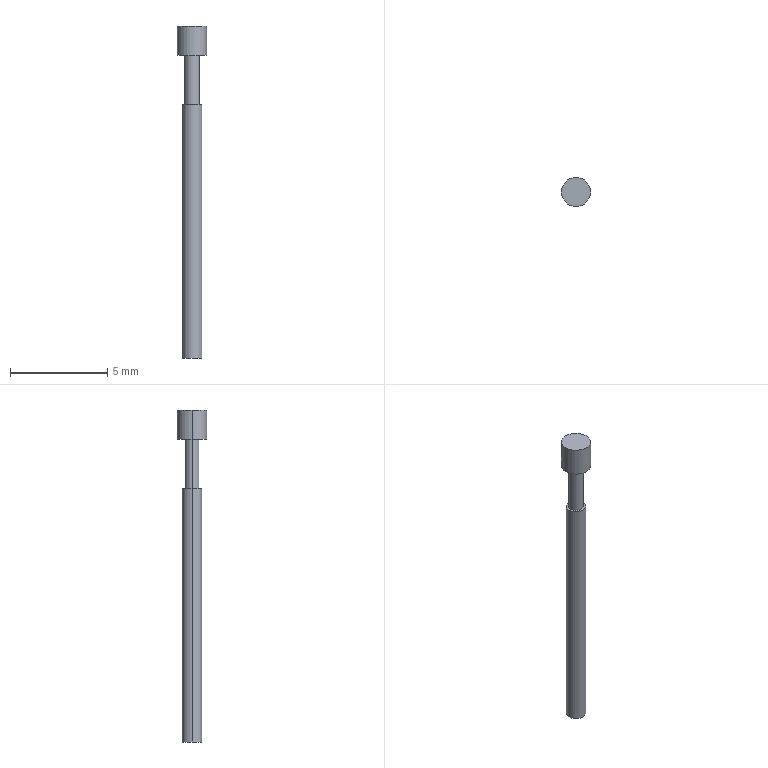Part | 1 solid | 10 faces | box 1.5 x 1.5 x 17.04 mm | volume 14.249 mm3 | cylinder 6 | plane 4 | commonest cylinder face diameters 0.77 x2 1.01 x2 1.5 x2
STEP:
#1=CARTESIAN_POINT('',(1988.973,168.494,-170.));
#2=VERTEX_POINT('',#1);
#3=CARTESIAN_POINT('',(1987.473,168.494,-170.));
#4=VERTEX_POINT('',#3);
#5=CARTESIAN_POINT('',(1988.223,168.494,-170.));
#6=DIRECTION('',(0.,0.,-1.));
#7=DIRECTION('',(-1.,0.,0.));
#8=AXIS2_PLACEMENT_3D('',#5,#6,#7);
#9=CIRCLE('',#8,0.75);
#10=EDGE_CURVE('',#2,#4,#9,.T.);
#11=ORIENTED_EDGE('',*,*,#10,.F.);
#12=CARTESIAN_POINT('',(1988.973,168.494,-168.5));
#13=VERTEX_POINT('',#12);
#14=CARTESIAN_POINT('',(1988.973,168.494,-168.5));
#15=DIRECTION('',(0.,0.,-1.));
#16=VECTOR('',#15,1000.);
#17=LINE('',#14,#16);
#18=EDGE_CURVE('',#2,#13,#17,.F.);
#19=ORIENTED_EDGE('',*,*,#18,.T.);
#20=CARTESIAN_POINT('',(1987.473,168.494,-168.5));
#21=VERTEX_POINT('',#20);
#22=CARTESIAN_POINT('',(1988.223,168.494,-168.5));
#23=DIRECTION('',(0.,0.,-1.));
#24=DIRECTION('',(-1.,0.,0.));
#25=AXIS2_PLACEMENT_3D('',#22,#23,#24);
#26=CIRCLE('',#25,0.75);
#27=EDGE_CURVE('',#13,#21,#26,.T.);
#28=ORIENTED_EDGE('',*,*,#27,.T.);
#29=CARTESIAN_POINT('',(1987.473,168.494,-168.5));
#30=DIRECTION('',(0.,0.,-1.));
#31=VECTOR('',#30,1000.);
#32=LINE('',#29,#31);
#33=EDGE_CURVE('',#4,#21,#32,.F.);
#34=ORIENTED_EDGE('',*,*,#33,.F.);
#35=EDGE_LOOP('',(#11,#19,#28,#34));
#36=FACE_BOUND('',#35,.T.);
#37=CARTESIAN_POINT('',(1988.223,168.494,-168.5));
#38=DIRECTION('',(0.,0.,-1.));
#39=DIRECTION('',(-1.,0.,0.));
#40=AXIS2_PLACEMENT_3D('',#37,#38,#39);
#41=CYLINDRICAL_SURFACE('',#40,0.75);
#42=ADVANCED_FACE('',(#36),#41,.T.);
#43=ORIENTED_EDGE('',*,*,#33,.T.);
#44=CARTESIAN_POINT('',(1988.223,168.494,-168.5));
#45=DIRECTION('',(0.,0.,-1.));
#46=DIRECTION('',(-1.,0.,0.));
#47=AXIS2_PLACEMENT_3D('',#44,#45,#46);
#48=CIRCLE('',#47,0.75);
#49=EDGE_CURVE('',#21,#13,#48,.T.);
#50=ORIENTED_EDGE('',*,*,#49,.T.);
#51=ORIENTED_EDGE('',*,*,#18,.F.);
#52=CARTESIAN_POINT('',(1988.223,168.494,-170.));
#53=DIRECTION('',(0.,0.,-1.));
#54=DIRECTION('',(-1.,0.,0.));
#55=AXIS2_PLACEMENT_3D('',#52,#53,#54);
#56=CIRCLE('',#55,0.75);
#57=EDGE_CURVE('',#4,#2,#56,.T.);
#58=ORIENTED_EDGE('',*,*,#57,.F.);
#59=EDGE_LOOP('',(#43,#50,#51,#58));
#60=FACE_BOUND('',#59,.T.);
#61=CARTESIAN_POINT('',(1988.223,168.494,-168.5));
#62=DIRECTION('',(0.,0.,-1.));
#63=DIRECTION('',(-1.,0.,0.));
#64=AXIS2_PLACEMENT_3D('',#61,#62,#63);
#65=CYLINDRICAL_SURFACE('',#64,0.75);
#66=ADVANCED_FACE('',(#60),#65,.T.);
#67=ORIENTED_EDGE('',*,*,#10,.T.);
#68=ORIENTED_EDGE('',*,*,#57,.T.);
#69=EDGE_LOOP('',(#67,#68));
#70=FACE_BOUND('',#69,.T.);
#71=CARTESIAN_POINT('',(1988.608,168.494,-170.));
#72=VERTEX_POINT('',#71);
#73=CARTESIAN_POINT('',(1987.838,168.494,-170.));
#74=VERTEX_POINT('',#73);
#75=CARTESIAN_POINT('',(1988.223,168.494,-170.));
#76=DIRECTION('',(0.,0.,-1.));
#77=DIRECTION('',(-1.,0.,0.));
#78=AXIS2_PLACEMENT_3D('',#75,#76,#77);
#79=CIRCLE('',#78,0.385);
#80=EDGE_CURVE('',#72,#74,#79,.T.);
#81=ORIENTED_EDGE('',*,*,#80,.F.);
#82=CARTESIAN_POINT('',(1988.223,168.494,-170.));
#83=DIRECTION('',(0.,0.,-1.));
#84=DIRECTION('',(-1.,0.,0.));
#85=AXIS2_PLACEMENT_3D('',#82,#83,#84);
#86=CIRCLE('',#85,0.385);
#87=EDGE_CURVE('',#74,#72,#86,.T.);
#88=ORIENTED_EDGE('',*,*,#87,.F.);
#89=EDGE_LOOP('',(#81,#88));
#90=FACE_BOUND('',#89,.T.);
#91=CARTESIAN_POINT('',(1990.223,166.494,-170.));
#92=DIRECTION('',(0.,0.,-1.));
#93=DIRECTION('',(0.,-1.,0.));
#94=AXIS2_PLACEMENT_3D('',#91,#92,#93);
#95=PLANE('',#94);
#96=ADVANCED_FACE('',(#70,#90),#95,.T.);
#97=CARTESIAN_POINT('',(1988.608,168.494,-172.54));
#98=VERTEX_POINT('',#97);
#99=CARTESIAN_POINT('',(1987.838,168.494,-172.54));
#100=VERTEX_POINT('',#99);
#101=CARTESIAN_POINT('',(1988.223,168.494,-172.54));
#102=DIRECTION('',(0.,0.,-1.));
#103=DIRECTION('',(-1.,0.,0.));
#104=AXIS2_PLACEMENT_3D('',#101,#102,#103);
#105=CIRCLE('',#104,0.385);
#106=EDGE_CURVE('',#98,#100,#105,.T.);
#107=ORIENTED_EDGE('',*,*,#106,.F.);
#108=CARTESIAN_POINT('',(1988.608,168.494,-170.));
#109=DIRECTION('',(0.,0.,-1.));
#110=VECTOR('',#109,1000.);
#111=LINE('',#108,#110);
#112=EDGE_CURVE('',#98,#72,#111,.F.);
#113=ORIENTED_EDGE('',*,*,#112,.T.);
#114=ORIENTED_EDGE('',*,*,#80,.T.);
#115=CARTESIAN_POINT('',(1987.838,168.494,-170.));
#116=DIRECTION('',(0.,0.,-1.));
#117=VECTOR('',#116,1000.);
#118=LINE('',#115,#117);
#119=EDGE_CURVE('',#100,#74,#118,.F.);
#120=ORIENTED_EDGE('',*,*,#119,.F.);
#121=EDGE_LOOP('',(#107,#113,#114,#120));
#122=FACE_BOUND('',#121,.T.);
#123=CARTESIAN_POINT('',(1988.223,168.494,-170.));
#124=DIRECTION('',(0.,0.,-1.));
#125=DIRECTION('',(-1.,0.,0.));
#126=AXIS2_PLACEMENT_3D('',#123,#124,#125);
#127=CYLINDRICAL_SURFACE('',#126,0.385);
#128=ADVANCED_FACE('',(#122),#127,.T.);
#129=CARTESIAN_POINT('',(1988.728,168.494,-172.54));
#130=VERTEX_POINT('',#129);
#131=CARTESIAN_POINT('',(1987.718,168.494,-172.54));
#132=VERTEX_POINT('',#131);
#133=CARTESIAN_POINT('',(1988.223,168.494,-172.54));
#134=DIRECTION('',(0.,0.,-1.));
#135=DIRECTION('',(-1.,0.,0.));
#136=AXIS2_PLACEMENT_3D('',#133,#134,#135);
#137=CIRCLE('',#136,0.505);
#138=EDGE_CURVE('',#130,#132,#137,.T.);
#139=ORIENTED_EDGE('',*,*,#138,.F.);
#140=CARTESIAN_POINT('',(1988.223,168.494,-172.54));
#141=DIRECTION('',(0.,0.,-1.));
#142=DIRECTION('',(-1.,0.,0.));
#143=AXIS2_PLACEMENT_3D('',#140,#141,#142);
#144=CIRCLE('',#143,0.505);
#145=EDGE_CURVE('',#132,#130,#144,.T.);
#146=ORIENTED_EDGE('',*,*,#145,.F.);
#147=EDGE_LOOP('',(#139,#146));
#148=FACE_BOUND('',#147,.T.);
#149=ORIENTED_EDGE('',*,*,#106,.T.);
#150=CARTESIAN_POINT('',(1988.223,168.494,-172.54));
#151=DIRECTION('',(0.,0.,-1.));
#152=DIRECTION('',(-1.,0.,0.));
#153=AXIS2_PLACEMENT_3D('',#150,#151,#152);
#154=CIRCLE('',#153,0.385);
#155=EDGE_CURVE('',#100,#98,#154,.T.);
#156=ORIENTED_EDGE('',*,*,#155,.T.);
#157=EDGE_LOOP('',(#149,#156));
#158=FACE_BOUND('',#157,.T.);
#159=CARTESIAN_POINT('',(1988.093,168.395,-172.54));
#160=DIRECTION('',(0.,0.,-1.));
#161=DIRECTION('',(0.,-1.,0.));
#162=AXIS2_PLACEMENT_3D('',#159,#160,#161);
#163=PLANE('',#162);
#164=ADVANCED_FACE('',(#148,#158),#163,.F.);
#165=CARTESIAN_POINT('',(1988.728,168.494,-185.54));
#166=VERTEX_POINT('',#165);
#167=CARTESIAN_POINT('',(1987.718,168.494,-185.54));
#168=VERTEX_POINT('',#167);
#169=CARTESIAN_POINT('',(1988.223,168.494,-185.54));
#170=DIRECTION('',(0.,0.,-1.));
#171=DIRECTION('',(-1.,0.,0.));
#172=AXIS2_PLACEMENT_3D('',#169,#170,#171);
#173=CIRCLE('',#172,0.505);
#174=EDGE_CURVE('',#166,#168,#173,.T.);
#175=ORIENTED_EDGE('',*,*,#174,.F.);
#176=CARTESIAN_POINT('',(1988.728,168.494,-172.54));
#177=DIRECTION('',(0.,0.,-1.));
#178=VECTOR('',#177,1000.);
#179=LINE('',#176,#178);
#180=EDGE_CURVE('',#166,#130,#179,.F.);
#181=ORIENTED_EDGE('',*,*,#180,.T.);
#182=ORIENTED_EDGE('',*,*,#138,.T.);
#183=CARTESIAN_POINT('',(1987.718,168.494,-172.54));
#184=DIRECTION('',(0.,0.,-1.));
#185=VECTOR('',#184,1000.);
#186=LINE('',#183,#185);
#187=EDGE_CURVE('',#168,#132,#186,.F.);
#188=ORIENTED_EDGE('',*,*,#187,.F.);
#189=EDGE_LOOP('',(#175,#181,#182,#188));
#190=FACE_BOUND('',#189,.T.);
#191=CARTESIAN_POINT('',(1988.223,168.494,-172.54));
#192=DIRECTION('',(0.,0.,-1.));
#193=DIRECTION('',(-1.,0.,0.));
#194=AXIS2_PLACEMENT_3D('',#191,#192,#193);
#195=CYLINDRICAL_SURFACE('',#194,0.505);
#196=ADVANCED_FACE('',(#190),#195,.T.);
#197=ORIENTED_EDGE('',*,*,#174,.T.);
#198=CARTESIAN_POINT('',(1988.223,168.494,-185.54));
#199=DIRECTION('',(0.,0.,-1.));
#200=DIRECTION('',(-1.,0.,0.));
#201=AXIS2_PLACEMENT_3D('',#198,#199,#200);
#202=CIRCLE('',#201,0.505);
#203=EDGE_CURVE('',#168,#166,#202,.T.);
#204=ORIENTED_EDGE('',*,*,#203,.T.);
#205=EDGE_LOOP('',(#197,#204));
#206=FACE_BOUND('',#205,.T.);
#207=CARTESIAN_POINT('',(1988.093,168.395,-185.54));
#208=DIRECTION('',(0.,0.,-1.));
#209=DIRECTION('',(0.,-1.,0.));
#210=AXIS2_PLACEMENT_3D('',#207,#208,#209);
#211=PLANE('',#210);
#212=ADVANCED_FACE('',(#206),#211,.T.);
#213=ORIENTED_EDGE('',*,*,#119,.T.);
#214=ORIENTED_EDGE('',*,*,#87,.T.);
#215=ORIENTED_EDGE('',*,*,#112,.F.);
#216=ORIENTED_EDGE('',*,*,#155,.F.);
#217=EDGE_LOOP('',(#213,#214,#215,#216));
#218=FACE_BOUND('',#217,.T.);
#219=CARTESIAN_POINT('',(1988.223,168.494,-170.));
#220=DIRECTION('',(0.,0.,-1.));
#221=DIRECTION('',(-1.,0.,0.));
#222=AXIS2_PLACEMENT_3D('',#219,#220,#221);
#223=CYLINDRICAL_SURFACE('',#222,0.385);
#224=ADVANCED_FACE('',(#218),#223,.T.);
#225=ORIENTED_EDGE('',*,*,#187,.T.);
#226=ORIENTED_EDGE('',*,*,#145,.T.);
#227=ORIENTED_EDGE('',*,*,#180,.F.);
#228=ORIENTED_EDGE('',*,*,#203,.F.);
#229=EDGE_LOOP('',(#225,#226,#227,#228));
#230=FACE_BOUND('',#229,.T.);
#231=CARTESIAN_POINT('',(1988.223,168.494,-172.54));
#232=DIRECTION('',(0.,0.,-1.));
#233=DIRECTION('',(-1.,0.,0.));
#234=AXIS2_PLACEMENT_3D('',#231,#232,#233);
#235=CYLINDRICAL_SURFACE('',#234,0.505);
#236=ADVANCED_FACE('',(#230),#235,.T.);
#237=ORIENTED_EDGE('',*,*,#27,.F.);
#238=ORIENTED_EDGE('',*,*,#49,.F.);
#239=EDGE_LOOP('',(#237,#238));
#240=FACE_BOUND('',#239,.T.);
#241=CARTESIAN_POINT('',(1990.223,166.494,-168.5));
#242=DIRECTION('',(0.,0.,-1.));
#243=DIRECTION('',(0.,-1.,0.));
#244=AXIS2_PLACEMENT_3D('',#241,#242,#243);
#245=PLANE('',#244);
#246=ADVANCED_FACE('',(#240),#245,.F.);
#247=CLOSED_SHELL('',(#42,#66,#96,#128,#164,#196,#212,#224,#236,#246));
#248=MANIFOLD_SOLID_BREP('',#247);
#249=(LENGTH_UNIT()NAMED_UNIT(*)SI_UNIT(.MILLI.,.METRE.));
#250=UNCERTAINTY_MEASURE_WITH_UNIT(LENGTH_MEASURE(0.00001),#249,'','');
#251=(NAMED_UNIT(*)PLANE_ANGLE_UNIT()SI_UNIT($,.RADIAN.));
#252=(NAMED_UNIT(*)SI_UNIT($,.STERADIAN.)SOLID_ANGLE_UNIT());
#253=(GEOMETRIC_REPRESENTATION_CONTEXT(3)GLOBAL_UNCERTAINTY_ASSIGNED_CONTEXT((#250))GLOBAL_UNIT_ASSIGNED_CONTEXT((#249,#251,#252))REPRESENTATION_CONTEXT('',''));
#254=ADVANCED_BREP_SHAPE_REPRESENTATION('',(#248),#253);